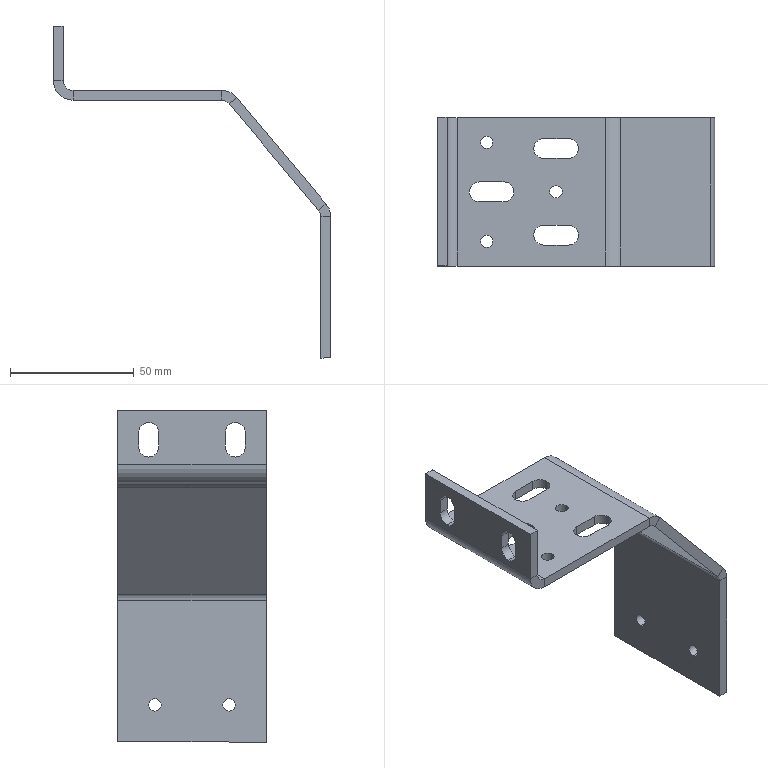Part | SolidWorks | features EdgeFlange 3, HoleWzd 2, ICE 2, FlatPattern 1, SMBaseFlange 1, SheetMetal 1 | 1 solid | 65 faces | box 112.169 x 60 x 134.193 mm | volume 48668 mm3 | plane 34 | cylinder 31 | commonest cylinder face diameters 8 x18 5 x10 16 x3